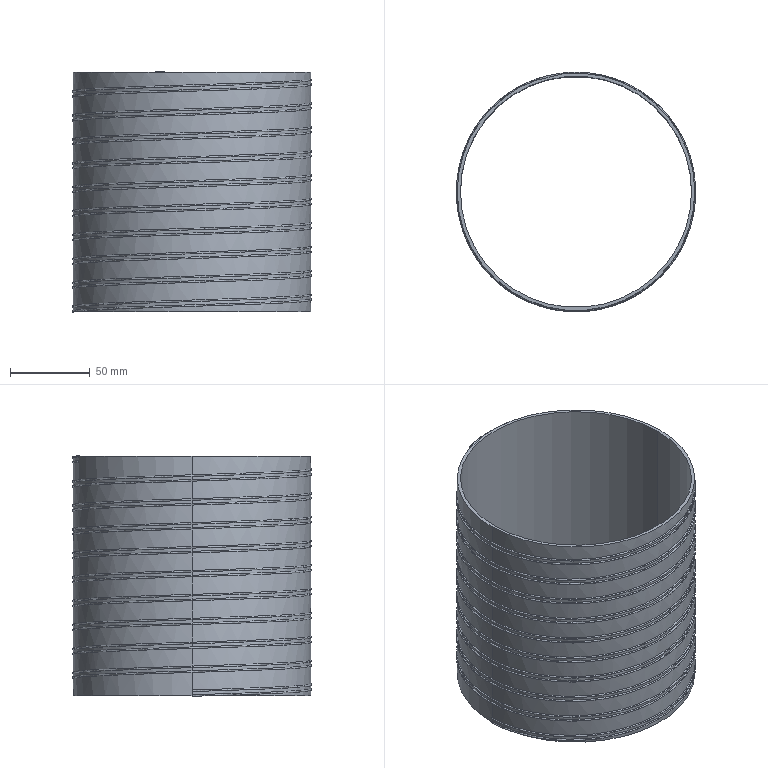Part | STEP file | D1450001 | 1 solid | 53 faces | box 150 x 150 x 151 mm | volume 142143 mm3 | cylinder 41 | plane 6 | spline 6 | commonest cylinder face diameters 149 x39 145 x2